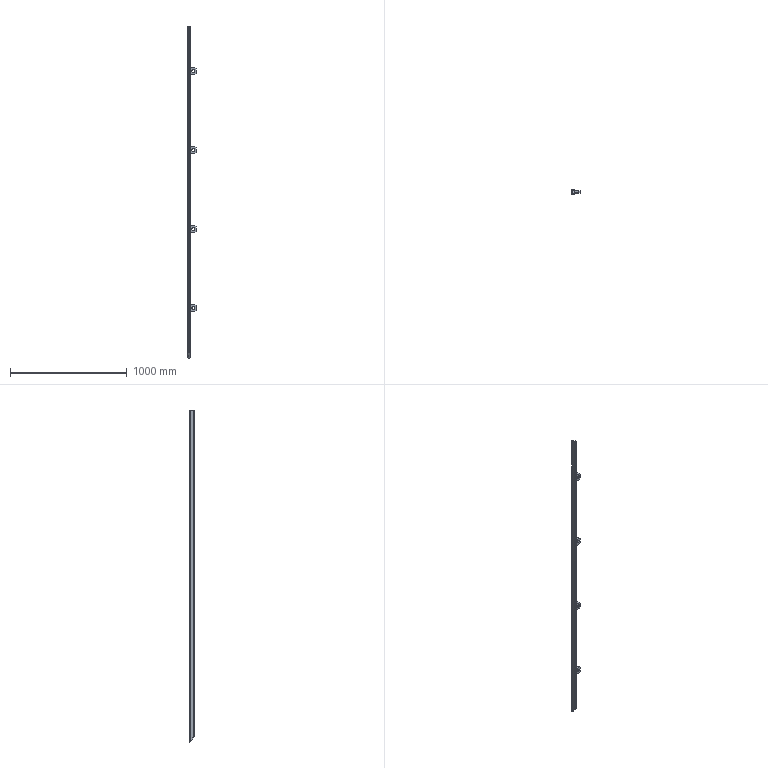Part | STEP file | 2 solids | 89 faces | box 70 x 40 x 2839 mm | volume 801093 mm3 | plane 44 | cylinder 29 | spline 8 | cone 8 | commonest cylinder face diameters 6.8 x8 26 x8 1 x5 2 x4 6 x4